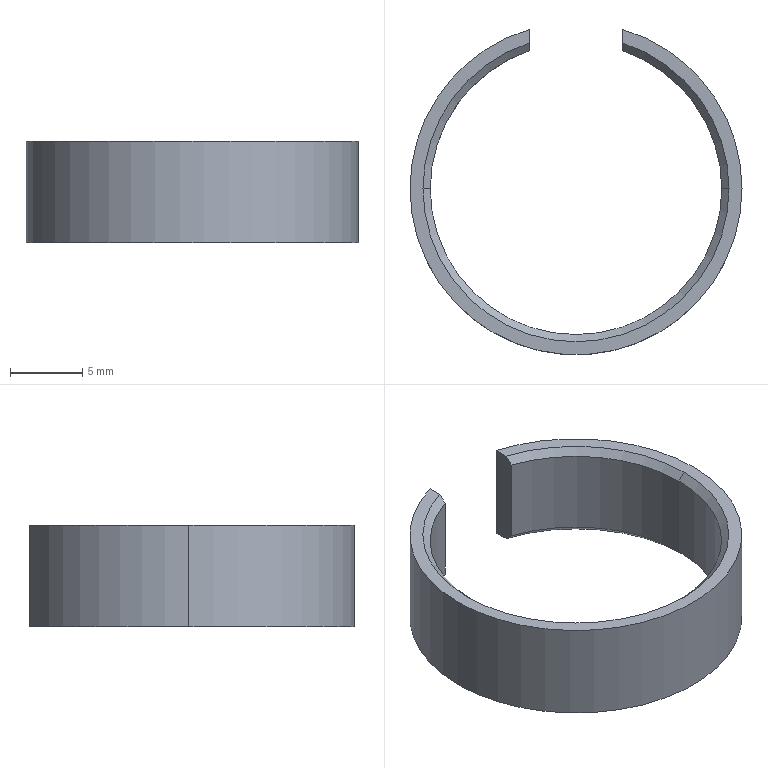Part | SolidWorks | features Chamfer 1, Extrusion 1, ICE 1 | 1 solid | 16 faces | box 23 x 22.531 x 7 mm | volume 585.831 mm3 | cone 6 | cylinder 6 | plane 4 | commonest cylinder face diameters 20.2 x3 23 x3
STEP:
#1=CARTESIAN_POINT('',(-10.1,0.,6.5));
#2=VERTEX_POINT('',#1);
#3=CARTESIAN_POINT('',(10.1,0.,6.5));
#4=VERTEX_POINT('',#3);
#5=CARTESIAN_POINT('',(0.,0.,6.5));
#6=DIRECTION('',(0.,0.,1.));
#7=DIRECTION('',(1.,0.,0.));
#8=AXIS2_PLACEMENT_3D('',#5,#6,#7);
#9=CIRCLE('',#8,10.1);
#10=EDGE_CURVE('',#2,#4,#9,.T.);
#11=ORIENTED_EDGE('',*,*,#10,.F.);
#12=CARTESIAN_POINT('',(-10.6,0.,7.));
#13=VERTEX_POINT('',#12);
#14=CARTESIAN_POINT('',(-10.1,0.,6.5));
#15=DIRECTION('',(-0.7071,0.,0.7071));
#16=VECTOR('',#15,1000.);
#17=LINE('',#14,#16);
#18=EDGE_CURVE('',#2,#13,#17,.T.);
#19=ORIENTED_EDGE('',*,*,#18,.T.);
#20=CARTESIAN_POINT('',(10.6,0.,7.));
#21=VERTEX_POINT('',#20);
#22=CARTESIAN_POINT('',(0.,0.,7.));
#23=DIRECTION('',(0.,0.,-1.));
#24=DIRECTION('',(1.,0.,0.));
#25=AXIS2_PLACEMENT_3D('',#22,#23,#24);
#26=CIRCLE('',#25,10.6);
#27=EDGE_CURVE('',#21,#13,#26,.T.);
#28=ORIENTED_EDGE('',*,*,#27,.F.);
#29=CARTESIAN_POINT('',(10.1,0.,6.5));
#30=DIRECTION('',(0.7071,0.,0.7071));
#31=VECTOR('',#30,1000.);
#32=LINE('',#29,#31);
#33=EDGE_CURVE('',#4,#21,#32,.T.);
#34=ORIENTED_EDGE('',*,*,#33,.F.);
#35=EDGE_LOOP('',(#11,#19,#28,#34));
#36=FACE_OUTER_BOUND('',#35,.T.);
#37=CARTESIAN_POINT('',(0.,0.,6.5));
#38=DIRECTION('',(0.,0.,1.));
#39=DIRECTION('',(1.,0.,0.));
#40=AXIS2_PLACEMENT_3D('',#37,#38,#39);
#41=CONICAL_SURFACE('',#40,10.1,0.7854);
#42=ADVANCED_FACE('',(#36),#41,.F.);
#43=CARTESIAN_POINT('',(3.25,9.563,6.5));
#44=VERTEX_POINT('',#43);
#45=CARTESIAN_POINT('',(0.,0.,6.5));
#46=DIRECTION('',(0.,0.,1.));
#47=DIRECTION('',(1.,0.,0.));
#48=AXIS2_PLACEMENT_3D('',#45,#46,#47);
#49=CIRCLE('',#48,10.1);
#50=EDGE_CURVE('',#4,#44,#49,.T.);
#51=ORIENTED_EDGE('',*,*,#50,.F.);
#52=ORIENTED_EDGE('',*,*,#33,.T.);
#53=CARTESIAN_POINT('',(3.25,10.089,7.));
#54=VERTEX_POINT('',#53);
#55=CARTESIAN_POINT('',(0.,0.,7.));
#56=DIRECTION('',(0.,0.,-1.));
#57=DIRECTION('',(1.,0.,0.));
#58=AXIS2_PLACEMENT_3D('',#55,#56,#57);
#59=CIRCLE('',#58,10.6);
#60=EDGE_CURVE('',#54,#21,#59,.T.);
#61=ORIENTED_EDGE('',*,*,#60,.F.);
#62=CARTESIAN_POINT('',(3.25,9.563,6.5));
#63=CARTESIAN_POINT('',(3.25,9.739,6.666));
#64=CARTESIAN_POINT('',(3.25,9.914,6.833));
#65=CARTESIAN_POINT('',(3.25,10.089,7.));
#66=B_SPLINE_CURVE_WITH_KNOTS('',3,(#62,#63,#64,#65),.UNSPECIFIED.,.F.,.F.,(4,4),(0.,0.0007262),.UNSPECIFIED.);
#67=EDGE_CURVE('',#44,#54,#66,.T.);
#68=ORIENTED_EDGE('',*,*,#67,.F.);
#69=EDGE_LOOP('',(#51,#52,#61,#68));
#70=FACE_OUTER_BOUND('',#69,.T.);
#71=CARTESIAN_POINT('',(0.,0.,6.5));
#72=DIRECTION('',(0.,0.,1.));
#73=DIRECTION('',(1.,0.,0.));
#74=AXIS2_PLACEMENT_3D('',#71,#72,#73);
#75=CONICAL_SURFACE('',#74,10.1,0.7854);
#76=ADVANCED_FACE('',(#70),#75,.F.);
#77=CARTESIAN_POINT('',(10.1,0.,0.5));
#78=VERTEX_POINT('',#77);
#79=CARTESIAN_POINT('',(-10.1,0.,0.5));
#80=VERTEX_POINT('',#79);
#81=CARTESIAN_POINT('',(0.,0.,0.5));
#82=DIRECTION('',(0.,0.,-1.));
#83=DIRECTION('',(1.,0.,0.));
#84=AXIS2_PLACEMENT_3D('',#81,#82,#83);
#85=CIRCLE('',#84,10.1);
#86=EDGE_CURVE('',#78,#80,#85,.T.);
#87=ORIENTED_EDGE('',*,*,#86,.F.);
#88=CARTESIAN_POINT('',(10.6,0.,0.));
#89=VERTEX_POINT('',#88);
#90=CARTESIAN_POINT('',(10.6,0.,0.));
#91=DIRECTION('',(0.7071,0.,-0.7071));
#92=VECTOR('',#91,1000.);
#93=LINE('',#90,#92);
#94=EDGE_CURVE('',#78,#89,#93,.T.);
#95=ORIENTED_EDGE('',*,*,#94,.T.);
#96=CARTESIAN_POINT('',(-10.6,0.,0.));
#97=VERTEX_POINT('',#96);
#98=CARTESIAN_POINT('',(0.,0.,0.));
#99=DIRECTION('',(0.,0.,1.));
#100=DIRECTION('',(1.,0.,0.));
#101=AXIS2_PLACEMENT_3D('',#98,#99,#100);
#102=CIRCLE('',#101,10.6);
#103=EDGE_CURVE('',#97,#89,#102,.T.);
#104=ORIENTED_EDGE('',*,*,#103,.F.);
#105=CARTESIAN_POINT('',(-10.6,0.,0.));
#106=DIRECTION('',(-0.7071,0.,-0.7071));
#107=VECTOR('',#106,1000.);
#108=LINE('',#105,#107);
#109=EDGE_CURVE('',#80,#97,#108,.T.);
#110=ORIENTED_EDGE('',*,*,#109,.F.);
#111=EDGE_LOOP('',(#87,#95,#104,#110));
#112=FACE_OUTER_BOUND('',#111,.T.);
#113=CARTESIAN_POINT('',(0.,0.,0.));
#114=DIRECTION('',(0.,0.,-1.));
#115=DIRECTION('',(-1.,0.,0.));
#116=AXIS2_PLACEMENT_3D('',#113,#114,#115);
#117=CONICAL_SURFACE('',#116,10.6,0.7854);
#118=ADVANCED_FACE('',(#112),#117,.F.);
#119=CARTESIAN_POINT('',(-3.25,9.563,0.5));
#120=VERTEX_POINT('',#119);
#121=CARTESIAN_POINT('',(0.,0.,0.5));
#122=DIRECTION('',(0.,0.,-1.));
#123=DIRECTION('',(1.,0.,0.));
#124=AXIS2_PLACEMENT_3D('',#121,#122,#123);
#125=CIRCLE('',#124,10.1);
#126=EDGE_CURVE('',#80,#120,#125,.T.);
#127=ORIENTED_EDGE('',*,*,#126,.F.);
#128=ORIENTED_EDGE('',*,*,#109,.T.);
#129=CARTESIAN_POINT('',(-3.25,10.089,0.));
#130=VERTEX_POINT('',#129);
#131=CARTESIAN_POINT('',(0.,0.,0.));
#132=DIRECTION('',(0.,0.,1.));
#133=DIRECTION('',(1.,0.,0.));
#134=AXIS2_PLACEMENT_3D('',#131,#132,#133);
#135=CIRCLE('',#134,10.6);
#136=EDGE_CURVE('',#130,#97,#135,.T.);
#137=ORIENTED_EDGE('',*,*,#136,.F.);
#138=CARTESIAN_POINT('',(-3.25,9.563,0.5));
#139=CARTESIAN_POINT('',(-3.25,9.739,0.3336));
#140=CARTESIAN_POINT('',(-3.25,9.914,0.1669));
#141=CARTESIAN_POINT('',(-3.25,10.089,0.));
#142=B_SPLINE_CURVE_WITH_KNOTS('',3,(#138,#139,#140,#141),.UNSPECIFIED.,.F.,.F.,(4,4),(0.,0.0007262),.UNSPECIFIED.);
#143=EDGE_CURVE('',#120,#130,#142,.T.);
#144=ORIENTED_EDGE('',*,*,#143,.F.);
#145=EDGE_LOOP('',(#127,#128,#137,#144));
#146=FACE_OUTER_BOUND('',#145,.T.);
#147=CARTESIAN_POINT('',(0.,0.,0.));
#148=DIRECTION('',(0.,0.,-1.));
#149=DIRECTION('',(-1.,0.,0.));
#150=AXIS2_PLACEMENT_3D('',#147,#148,#149);
#151=CONICAL_SURFACE('',#150,10.6,0.7854);
#152=ADVANCED_FACE('',(#146),#151,.F.);
#153=ORIENTED_EDGE('',*,*,#10,.T.);
#154=CARTESIAN_POINT('',(10.1,0.,7.));
#155=DIRECTION('',(0.,0.,-1.));
#156=VECTOR('',#155,1000.);
#157=LINE('',#154,#156);
#158=EDGE_CURVE('',#4,#78,#157,.T.);
#159=ORIENTED_EDGE('',*,*,#158,.T.);
#160=ORIENTED_EDGE('',*,*,#86,.T.);
#161=CARTESIAN_POINT('',(-10.1,0.,7.));
#162=DIRECTION('',(0.,0.,-1.));
#163=VECTOR('',#162,1000.);
#164=LINE('',#161,#163);
#165=EDGE_CURVE('',#2,#80,#164,.T.);
#166=ORIENTED_EDGE('',*,*,#165,.F.);
#167=EDGE_LOOP('',(#153,#159,#160,#166));
#168=FACE_OUTER_BOUND('',#167,.T.);
#169=CARTESIAN_POINT('',(0.,0.,7.));
#170=DIRECTION('',(0.,0.,-1.));
#171=DIRECTION('',(-1.,0.,0.));
#172=AXIS2_PLACEMENT_3D('',#169,#170,#171);
#173=CYLINDRICAL_SURFACE('',#172,10.1);
#174=ADVANCED_FACE('',(#168),#173,.F.);
#175=CARTESIAN_POINT('',(-3.25,9.563,6.5));
#176=VERTEX_POINT('',#175);
#177=CARTESIAN_POINT('',(0.,0.,6.5));
#178=DIRECTION('',(0.,0.,1.));
#179=DIRECTION('',(1.,0.,0.));
#180=AXIS2_PLACEMENT_3D('',#177,#178,#179);
#181=CIRCLE('',#180,10.1);
#182=EDGE_CURVE('',#176,#2,#181,.T.);
#183=ORIENTED_EDGE('',*,*,#182,.T.);
#184=ORIENTED_EDGE('',*,*,#165,.T.);
#185=ORIENTED_EDGE('',*,*,#126,.T.);
#186=CARTESIAN_POINT('',(-3.25,9.563,7.));
#187=DIRECTION('',(0.,0.,-1.));
#188=VECTOR('',#187,1000.);
#189=LINE('',#186,#188);
#190=EDGE_CURVE('',#176,#120,#189,.T.);
#191=ORIENTED_EDGE('',*,*,#190,.F.);
#192=EDGE_LOOP('',(#183,#184,#185,#191));
#193=FACE_OUTER_BOUND('',#192,.T.);
#194=CARTESIAN_POINT('',(0.,0.,7.));
#195=DIRECTION('',(0.,0.,-1.));
#196=DIRECTION('',(-1.,0.,0.));
#197=AXIS2_PLACEMENT_3D('',#194,#195,#196);
#198=CYLINDRICAL_SURFACE('',#197,10.1);
#199=ADVANCED_FACE('',(#193),#198,.F.);
#200=CARTESIAN_POINT('',(11.5,0.,7.));
#201=VERTEX_POINT('',#200);
#202=CARTESIAN_POINT('',(3.25,11.031,7.));
#203=VERTEX_POINT('',#202);
#204=CARTESIAN_POINT('',(0.,0.,7.));
#205=DIRECTION('',(0.,0.,1.));
#206=DIRECTION('',(1.,0.,0.));
#207=AXIS2_PLACEMENT_3D('',#204,#205,#206);
#208=CIRCLE('',#207,11.5);
#209=EDGE_CURVE('',#201,#203,#208,.T.);
#210=ORIENTED_EDGE('',*,*,#209,.F.);
#211=CARTESIAN_POINT('',(11.5,0.,0.));
#212=VERTEX_POINT('',#211);
#213=CARTESIAN_POINT('',(11.5,0.,7.));
#214=DIRECTION('',(0.,0.,-1.));
#215=VECTOR('',#214,1000.);
#216=LINE('',#213,#215);
#217=EDGE_CURVE('',#201,#212,#216,.T.);
#218=ORIENTED_EDGE('',*,*,#217,.T.);
#219=CARTESIAN_POINT('',(3.25,11.031,0.));
#220=VERTEX_POINT('',#219);
#221=CARTESIAN_POINT('',(0.,0.,0.));
#222=DIRECTION('',(0.,0.,1.));
#223=DIRECTION('',(1.,0.,0.));
#224=AXIS2_PLACEMENT_3D('',#221,#222,#223);
#225=CIRCLE('',#224,11.5);
#226=EDGE_CURVE('',#212,#220,#225,.T.);
#227=ORIENTED_EDGE('',*,*,#226,.T.);
#228=CARTESIAN_POINT('',(3.25,11.031,7.));
#229=DIRECTION('',(0.,0.,1.));
#230=VECTOR('',#229,1000.);
#231=LINE('',#228,#230);
#232=EDGE_CURVE('',#220,#203,#231,.T.);
#233=ORIENTED_EDGE('',*,*,#232,.T.);
#234=EDGE_LOOP('',(#210,#218,#227,#233));
#235=FACE_OUTER_BOUND('',#234,.T.);
#236=CARTESIAN_POINT('',(0.,0.,7.));
#237=DIRECTION('',(0.,0.,-1.));
#238=DIRECTION('',(-1.,0.,0.));
#239=AXIS2_PLACEMENT_3D('',#236,#237,#238);
#240=CYLINDRICAL_SURFACE('',#239,11.5);
#241=ADVANCED_FACE('',(#235),#240,.T.);
#242=ORIENTED_EDGE('',*,*,#217,.F.);
#243=CARTESIAN_POINT('',(-11.5,0.,7.));
#244=VERTEX_POINT('',#243);
#245=CARTESIAN_POINT('',(0.,0.,7.));
#246=DIRECTION('',(0.,0.,1.));
#247=DIRECTION('',(1.,0.,0.));
#248=AXIS2_PLACEMENT_3D('',#245,#246,#247);
#249=CIRCLE('',#248,11.5);
#250=EDGE_CURVE('',#244,#201,#249,.T.);
#251=ORIENTED_EDGE('',*,*,#250,.F.);
#252=CARTESIAN_POINT('',(-11.5,0.,0.));
#253=VERTEX_POINT('',#252);
#254=CARTESIAN_POINT('',(-11.5,0.,7.));
#255=DIRECTION('',(0.,0.,-1.));
#256=VECTOR('',#255,1000.);
#257=LINE('',#254,#256);
#258=EDGE_CURVE('',#244,#253,#257,.T.);
#259=ORIENTED_EDGE('',*,*,#258,.T.);
#260=CARTESIAN_POINT('',(0.,0.,0.));
#261=DIRECTION('',(0.,0.,1.));
#262=DIRECTION('',(1.,0.,0.));
#263=AXIS2_PLACEMENT_3D('',#260,#261,#262);
#264=CIRCLE('',#263,11.5);
#265=EDGE_CURVE('',#253,#212,#264,.T.);
#266=ORIENTED_EDGE('',*,*,#265,.T.);
#267=EDGE_LOOP('',(#242,#251,#259,#266));
#268=FACE_OUTER_BOUND('',#267,.T.);
#269=CARTESIAN_POINT('',(0.,0.,7.));
#270=DIRECTION('',(0.,0.,-1.));
#271=DIRECTION('',(-1.,0.,0.));
#272=AXIS2_PLACEMENT_3D('',#269,#270,#271);
#273=CYLINDRICAL_SURFACE('',#272,11.5);
#274=ADVANCED_FACE('',(#268),#273,.T.);
#275=CARTESIAN_POINT('',(3.25,0.,7.));
#276=DIRECTION('',(0.,1.,0.));
#277=VECTOR('',#276,1000.);
#278=LINE('',#275,#277);
#279=EDGE_CURVE('',#54,#203,#278,.T.);
#280=ORIENTED_EDGE('',*,*,#279,.F.);
#281=ORIENTED_EDGE('',*,*,#60,.T.);
#282=ORIENTED_EDGE('',*,*,#27,.T.);
#283=CARTESIAN_POINT('',(-3.25,10.089,7.));
#284=VERTEX_POINT('',#283);
#285=CARTESIAN_POINT('',(0.,0.,7.));
#286=DIRECTION('',(0.,0.,-1.));
#287=DIRECTION('',(1.,0.,0.));
#288=AXIS2_PLACEMENT_3D('',#285,#286,#287);
#289=CIRCLE('',#288,10.6);
#290=EDGE_CURVE('',#13,#284,#289,.T.);
#291=ORIENTED_EDGE('',*,*,#290,.T.);
#292=CARTESIAN_POINT('',(-3.25,11.031,7.));
#293=VERTEX_POINT('',#292);
#294=CARTESIAN_POINT('',(-3.25,0.,7.));
#295=DIRECTION('',(0.,-1.,0.));
#296=VECTOR('',#295,1000.);
#297=LINE('',#294,#296);
#298=EDGE_CURVE('',#293,#284,#297,.T.);
#299=ORIENTED_EDGE('',*,*,#298,.F.);
#300=CARTESIAN_POINT('',(0.,0.,7.));
#301=DIRECTION('',(0.,0.,1.));
#302=DIRECTION('',(1.,0.,0.));
#303=AXIS2_PLACEMENT_3D('',#300,#301,#302);
#304=CIRCLE('',#303,11.5);
#305=EDGE_CURVE('',#293,#244,#304,.T.);
#306=ORIENTED_EDGE('',*,*,#305,.T.);
#307=ORIENTED_EDGE('',*,*,#250,.T.);
#308=ORIENTED_EDGE('',*,*,#209,.T.);
#309=EDGE_LOOP('',(#280,#281,#282,#291,#299,#306,#307,#308));
#310=FACE_OUTER_BOUND('',#309,.T.);
#311=CARTESIAN_POINT('',(0.,0.,7.));
#312=DIRECTION('',(0.,0.,1.));
#313=DIRECTION('',(1.,0.,0.));
#314=AXIS2_PLACEMENT_3D('',#311,#312,#313);
#315=PLANE('',#314);
#316=ADVANCED_FACE('',(#310),#315,.T.);
#317=CARTESIAN_POINT('',(-3.25,11.031,0.));
#318=VERTEX_POINT('',#317);
#319=CARTESIAN_POINT('',(-3.25,0.,0.));
#320=DIRECTION('',(0.,-1.,0.));
#321=VECTOR('',#320,1000.);
#322=LINE('',#319,#321);
#323=EDGE_CURVE('',#318,#130,#322,.T.);
#324=ORIENTED_EDGE('',*,*,#323,.T.);
#325=ORIENTED_EDGE('',*,*,#136,.T.);
#326=ORIENTED_EDGE('',*,*,#103,.T.);
#327=CARTESIAN_POINT('',(3.25,10.089,0.));
#328=VERTEX_POINT('',#327);
#329=CARTESIAN_POINT('',(0.,0.,0.));
#330=DIRECTION('',(0.,0.,1.));
#331=DIRECTION('',(1.,0.,0.));
#332=AXIS2_PLACEMENT_3D('',#329,#330,#331);
#333=CIRCLE('',#332,10.6);
#334=EDGE_CURVE('',#89,#328,#333,.T.);
#335=ORIENTED_EDGE('',*,*,#334,.T.);
#336=CARTESIAN_POINT('',(3.25,0.,0.));
#337=DIRECTION('',(0.,1.,0.));
#338=VECTOR('',#337,1000.);
#339=LINE('',#336,#338);
#340=EDGE_CURVE('',#328,#220,#339,.T.);
#341=ORIENTED_EDGE('',*,*,#340,.T.);
#342=ORIENTED_EDGE('',*,*,#226,.F.);
#343=ORIENTED_EDGE('',*,*,#265,.F.);
#344=CARTESIAN_POINT('',(0.,0.,0.));
#345=DIRECTION('',(0.,0.,1.));
#346=DIRECTION('',(1.,0.,0.));
#347=AXIS2_PLACEMENT_3D('',#344,#345,#346);
#348=CIRCLE('',#347,11.5);
#349=EDGE_CURVE('',#318,#253,#348,.T.);
#350=ORIENTED_EDGE('',*,*,#349,.F.);
#351=EDGE_LOOP('',(#324,#325,#326,#335,#341,#342,#343,#350));
#352=FACE_OUTER_BOUND('',#351,.T.);
#353=CARTESIAN_POINT('',(0.,0.,0.));
#354=DIRECTION('',(0.,0.,1.));
#355=DIRECTION('',(1.,0.,0.));
#356=AXIS2_PLACEMENT_3D('',#353,#354,#355);
#357=PLANE('',#356);
#358=ADVANCED_FACE('',(#352),#357,.F.);
#359=ORIENTED_EDGE('',*,*,#258,.F.);
#360=ORIENTED_EDGE('',*,*,#305,.F.);
#361=CARTESIAN_POINT('',(-3.25,11.031,7.));
#362=DIRECTION('',(0.,0.,-1.));
#363=VECTOR('',#362,1000.);
#364=LINE('',#361,#363);
#365=EDGE_CURVE('',#293,#318,#364,.T.);
#366=ORIENTED_EDGE('',*,*,#365,.T.);
#367=ORIENTED_EDGE('',*,*,#349,.T.);
#368=EDGE_LOOP('',(#359,#360,#366,#367));
#369=FACE_OUTER_BOUND('',#368,.T.);
#370=CARTESIAN_POINT('',(0.,0.,7.));
#371=DIRECTION('',(0.,0.,-1.));
#372=DIRECTION('',(-1.,0.,0.));
#373=AXIS2_PLACEMENT_3D('',#370,#371,#372);
#374=CYLINDRICAL_SURFACE('',#373,11.5);
#375=ADVANCED_FACE('',(#369),#374,.T.);
#376=ORIENTED_EDGE('',*,*,#158,.F.);
#377=ORIENTED_EDGE('',*,*,#50,.T.);
#378=CARTESIAN_POINT('',(3.25,9.563,0.5));
#379=VERTEX_POINT('',#378);
#380=CARTESIAN_POINT('',(3.25,9.563,7.));
#381=DIRECTION('',(0.,0.,1.));
#382=VECTOR('',#381,1000.);
#383=LINE('',#380,#382);
#384=EDGE_CURVE('',#379,#44,#383,.T.);
#385=ORIENTED_EDGE('',*,*,#384,.F.);
#386=CARTESIAN_POINT('',(0.,0.,0.5));
#387=DIRECTION('',(0.,0.,-1.));
#388=DIRECTION('',(1.,0.,0.));
#389=AXIS2_PLACEMENT_3D('',#386,#387,#388);
#390=CIRCLE('',#389,10.1);
#391=EDGE_CURVE('',#379,#78,#390,.T.);
#392=ORIENTED_EDGE('',*,*,#391,.T.);
#393=EDGE_LOOP('',(#376,#377,#385,#392));
#394=FACE_OUTER_BOUND('',#393,.T.);
#395=CARTESIAN_POINT('',(0.,0.,7.));
#396=DIRECTION('',(0.,0.,-1.));
#397=DIRECTION('',(-1.,0.,0.));
#398=AXIS2_PLACEMENT_3D('',#395,#396,#397);
#399=CYLINDRICAL_SURFACE('',#398,10.1);
#400=ADVANCED_FACE('',(#394),#399,.F.);
#401=ORIENTED_EDGE('',*,*,#340,.F.);
#402=CARTESIAN_POINT('',(3.25,10.089,0.));
#403=CARTESIAN_POINT('',(3.25,9.914,0.1669));
#404=CARTESIAN_POINT('',(3.25,9.739,0.3336));
#405=CARTESIAN_POINT('',(3.25,9.563,0.5));
#406=B_SPLINE_CURVE_WITH_KNOTS('',3,(#402,#403,#404,#405),.UNSPECIFIED.,.F.,.F.,(4,4),(0.,0.0007262),.UNSPECIFIED.);
#407=EDGE_CURVE('',#328,#379,#406,.T.);
#408=ORIENTED_EDGE('',*,*,#407,.T.);
#409=ORIENTED_EDGE('',*,*,#384,.T.);
#410=ORIENTED_EDGE('',*,*,#67,.T.);
#411=ORIENTED_EDGE('',*,*,#279,.T.);
#412=ORIENTED_EDGE('',*,*,#232,.F.);
#413=EDGE_LOOP('',(#401,#408,#409,#410,#411,#412));
#414=FACE_OUTER_BOUND('',#413,.T.);
#415=CARTESIAN_POINT('',(3.25,0.,0.));
#416=DIRECTION('',(1.,0.,0.));
#417=DIRECTION('',(0.,1.,0.));
#418=AXIS2_PLACEMENT_3D('',#415,#416,#417);
#419=PLANE('',#418);
#420=ADVANCED_FACE('',(#414),#419,.F.);
#421=ORIENTED_EDGE('',*,*,#190,.T.);
#422=ORIENTED_EDGE('',*,*,#143,.T.);
#423=ORIENTED_EDGE('',*,*,#323,.F.);
#424=ORIENTED_EDGE('',*,*,#365,.F.);
#425=ORIENTED_EDGE('',*,*,#298,.T.);
#426=CARTESIAN_POINT('',(-3.25,10.089,7.));
#427=CARTESIAN_POINT('',(-3.25,9.914,6.833));
#428=CARTESIAN_POINT('',(-3.25,9.739,6.666));
#429=CARTESIAN_POINT('',(-3.25,9.563,6.5));
#430=B_SPLINE_CURVE_WITH_KNOTS('',3,(#426,#427,#428,#429),.UNSPECIFIED.,.F.,.F.,(4,4),(0.,0.0007262),.UNSPECIFIED.);
#431=EDGE_CURVE('',#284,#176,#430,.T.);
#432=ORIENTED_EDGE('',*,*,#431,.T.);
#433=EDGE_LOOP('',(#421,#422,#423,#424,#425,#432));
#434=FACE_OUTER_BOUND('',#433,.T.);
#435=CARTESIAN_POINT('',(-3.25,0.,0.));
#436=DIRECTION('',(-1.,0.,0.));
#437=DIRECTION('',(0.,0.,1.));
#438=AXIS2_PLACEMENT_3D('',#435,#436,#437);
#439=PLANE('',#438);
#440=ADVANCED_FACE('',(#434),#439,.F.);
#441=ORIENTED_EDGE('',*,*,#94,.F.);
#442=ORIENTED_EDGE('',*,*,#391,.F.);
#443=ORIENTED_EDGE('',*,*,#407,.F.);
#444=ORIENTED_EDGE('',*,*,#334,.F.);
#445=EDGE_LOOP('',(#441,#442,#443,#444));
#446=FACE_OUTER_BOUND('',#445,.T.);
#447=CARTESIAN_POINT('',(0.,0.,0.));
#448=DIRECTION('',(0.,0.,-1.));
#449=DIRECTION('',(-1.,0.,0.));
#450=AXIS2_PLACEMENT_3D('',#447,#448,#449);
#451=CONICAL_SURFACE('',#450,10.6,0.7854);
#452=ADVANCED_FACE('',(#446),#451,.F.);
#453=ORIENTED_EDGE('',*,*,#18,.F.);
#454=ORIENTED_EDGE('',*,*,#182,.F.);
#455=ORIENTED_EDGE('',*,*,#431,.F.);
#456=ORIENTED_EDGE('',*,*,#290,.F.);
#457=EDGE_LOOP('',(#453,#454,#455,#456));
#458=FACE_OUTER_BOUND('',#457,.T.);
#459=CARTESIAN_POINT('',(0.,0.,6.5));
#460=DIRECTION('',(0.,0.,1.));
#461=DIRECTION('',(1.,0.,0.));
#462=AXIS2_PLACEMENT_3D('',#459,#460,#461);
#463=CONICAL_SURFACE('',#462,10.1,0.7854);
#464=ADVANCED_FACE('',(#458),#463,.F.);
#465=CLOSED_SHELL('',(#42,#76,#118,#152,#174,#199,#241,#274,#316,#358,#375,#400,#420,#440,#452,#464));
#466=MANIFOLD_SOLID_BREP('',#465);
#467=CARTESIAN_POINT('',(0.,0.,0.));
#468=DIRECTION('',(0.,0.,1.));
#469=DIRECTION('',(1.,0.,0.));
#470=AXIS2_PLACEMENT_3D('',#467,#468,#469);
#471=(LENGTH_UNIT()NAMED_UNIT(*)SI_UNIT(.MILLI.,.METRE.));
#472=UNCERTAINTY_MEASURE_WITH_UNIT(LENGTH_MEASURE(0.00001),#471,'','');
#473=(NAMED_UNIT(*)PLANE_ANGLE_UNIT()SI_UNIT($,.RADIAN.));
#474=(NAMED_UNIT(*)SI_UNIT($,.STERADIAN.)SOLID_ANGLE_UNIT());
#475=(GEOMETRIC_REPRESENTATION_CONTEXT(3)GLOBAL_UNCERTAINTY_ASSIGNED_CONTEXT((#472))GLOBAL_UNIT_ASSIGNED_CONTEXT((#471,#473,#474))REPRESENTATION_CONTEXT('',''));
#476=ADVANCED_BREP_SHAPE_REPRESENTATION('',(#466,#470),#475);